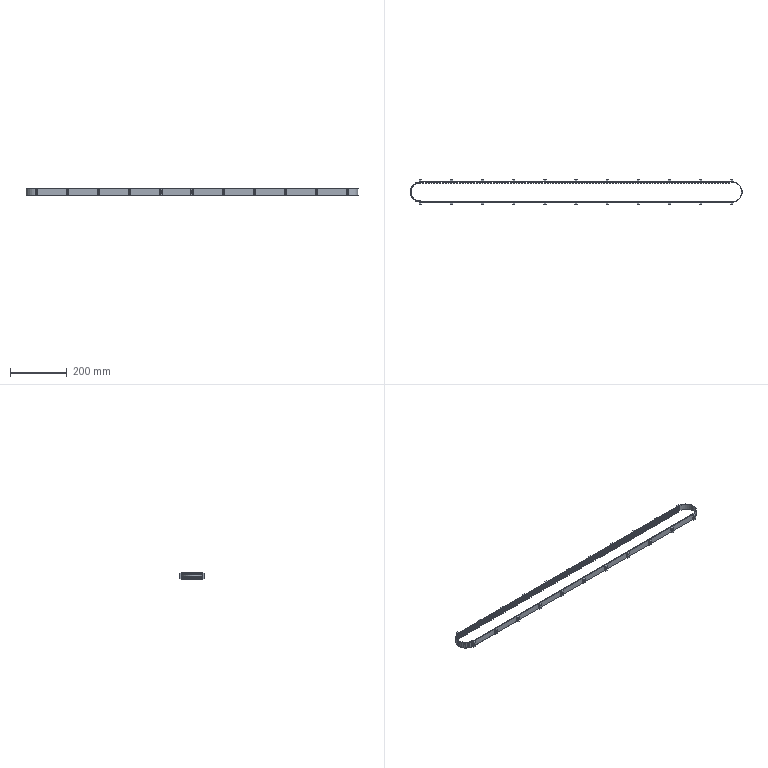Part | STEP file | Timing belt with stop block 2420-T10-21mm wide | 1 solid | 1284 faces | box 1172 x 86.18 x 21.9 mm | volume 158627 mm3 | cylinder 604 | plane 592 | cone 88 | commonest cylinder face diameters 1.6 x250 1.2 x242 2.5 x96 68.18 x13 72.18 x3